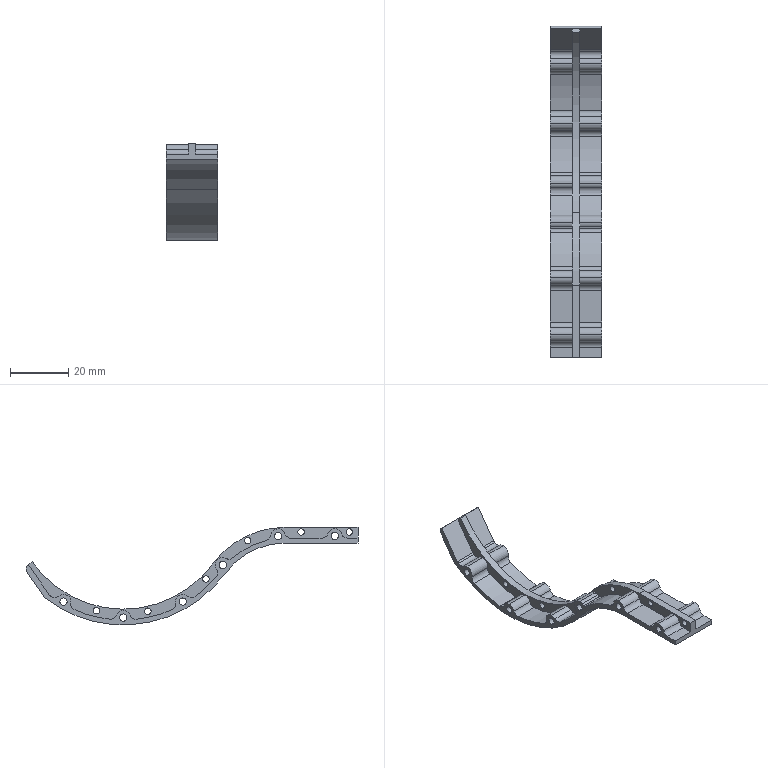Part | SolidWorks | features Extrusion 1, Fillet 1, HoleWzd 1, ICE 1 | 1 solid | 105 faces | box 17.6 x 113.917 x 33.473 mm | volume 5862 mm3 | cylinder 90 | plane 15 | commonest cylinder face diameters 4 x28 5 x24 2.2 x12 2.5 x12 83.6 x8 54.4 x2